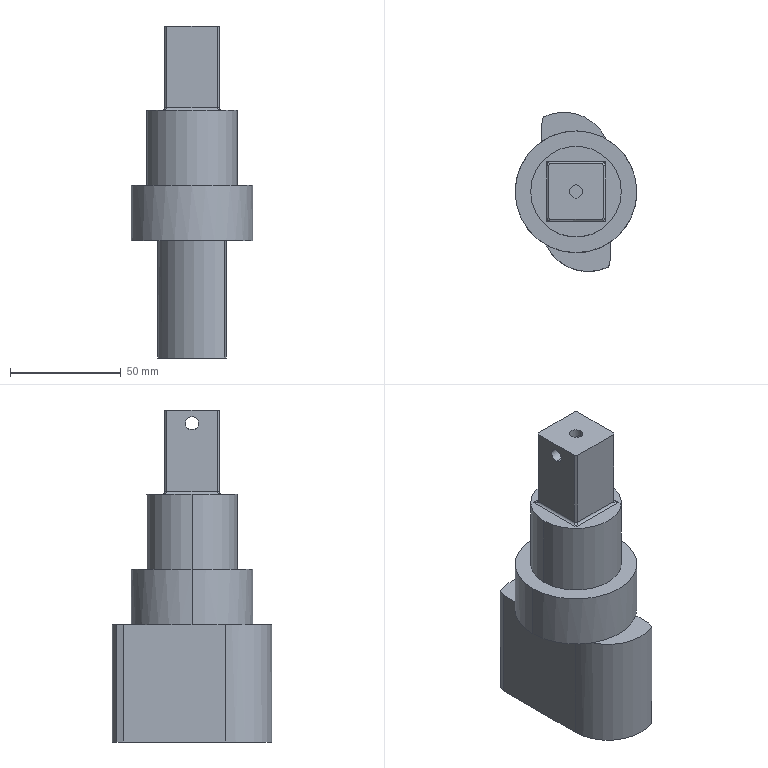Part | SolidWorks | features Boss 3, Chamfer 2, Cut 2, Extrusion 1, Fillet 1 | 1 solid | 43 faces | box 55 x 72 x 150 mm | volume 234412 mm3 | plane 21 | cylinder 18 | spline 4 | commonest cylinder face diameters 6 x8 2 x4 41 x2 42 x2 55 x2
STEP:
#1=CARTESIAN_POINT('',(-3.,0.,140.));
#2=VERTEX_POINT('',#1);
#3=CARTESIAN_POINT('',(3.,0.,140.));
#4=VERTEX_POINT('',#3);
#5=CARTESIAN_POINT('',(0.,0.,140.));
#6=DIRECTION('',(0.,0.,1.));
#7=DIRECTION('',(1.,0.,0.));
#8=AXIS2_PLACEMENT_3D('',#5,#6,#7);
#9=CIRCLE('',#8,3.);
#10=EDGE_CURVE('',#2,#4,#9,.T.);
#11=ORIENTED_EDGE('',*,*,#10,.F.);
#12=CARTESIAN_POINT('',(-3.,0.,141.));
#13=VERTEX_POINT('',#12);
#14=CARTESIAN_POINT('',(-3.,0.,140.));
#15=DIRECTION('',(0.,0.,1.));
#16=VECTOR('',#15,1000.);
#17=LINE('',#14,#16);
#18=EDGE_CURVE('',#2,#13,#17,.T.);
#19=ORIENTED_EDGE('',*,*,#18,.T.);
#20=CARTESIAN_POINT('',(0.,-3.,144.));
#21=VERTEX_POINT('',#20);
#22=CARTESIAN_POINT('',(0.,-3.,144.));
#23=CARTESIAN_POINT('',(-1.757,-3.,142.243));
#24=CARTESIAN_POINT('',(-3.,-1.757,141.));
#25=CARTESIAN_POINT('',(-3.,0.,141.));
#26=(BOUNDED_CURVE()B_SPLINE_CURVE(3,(#22,#23,#24,#25),.UNSPECIFIED.,.F.,.F.)B_SPLINE_CURVE_WITH_KNOTS((4,4),(4.712,6.283),.UNSPECIFIED.)CURVE()GEOMETRIC_REPRESENTATION_ITEM()RATIONAL_B_SPLINE_CURVE((1.,0.8047,0.8047,1.))REPRESENTATION_ITEM(''));
#27=EDGE_CURVE('',#21,#13,#26,.T.);
#28=ORIENTED_EDGE('',*,*,#27,.F.);
#29=CARTESIAN_POINT('',(3.,0.,141.));
#30=VERTEX_POINT('',#29);
#31=CARTESIAN_POINT('',(3.,0.,141.));
#32=CARTESIAN_POINT('',(3.,-1.757,141.));
#33=CARTESIAN_POINT('',(1.757,-3.,142.243));
#34=CARTESIAN_POINT('',(0.,-3.,144.));
#35=(BOUNDED_CURVE()B_SPLINE_CURVE(3,(#31,#32,#33,#34),.UNSPECIFIED.,.F.,.F.)B_SPLINE_CURVE_WITH_KNOTS((4,4),(3.142,4.712),.UNSPECIFIED.)CURVE()GEOMETRIC_REPRESENTATION_ITEM()RATIONAL_B_SPLINE_CURVE((1.,0.8047,0.8047,1.))REPRESENTATION_ITEM(''));
#36=EDGE_CURVE('',#30,#21,#35,.T.);
#37=ORIENTED_EDGE('',*,*,#36,.F.);
#38=CARTESIAN_POINT('',(3.,0.,140.));
#39=DIRECTION('',(0.,0.,1.));
#40=VECTOR('',#39,1000.);
#41=LINE('',#38,#40);
#42=EDGE_CURVE('',#4,#30,#41,.T.);
#43=ORIENTED_EDGE('',*,*,#42,.F.);
#44=EDGE_LOOP('',(#11,#19,#28,#37,#43));
#45=FACE_OUTER_BOUND('',#44,.T.);
#46=CARTESIAN_POINT('',(0.,0.,140.));
#47=DIRECTION('',(0.,0.,1.));
#48=DIRECTION('',(1.,0.,0.));
#49=AXIS2_PLACEMENT_3D('',#46,#47,#48);
#50=CYLINDRICAL_SURFACE('',#49,3.);
#51=ADVANCED_FACE('',(#45),#50,.F.);
#52=CARTESIAN_POINT('',(-3.,0.,147.));
#53=VERTEX_POINT('',#52);
#54=CARTESIAN_POINT('',(-3.,0.,147.));
#55=CARTESIAN_POINT('',(-3.,-1.757,147.));
#56=CARTESIAN_POINT('',(-1.757,-3.,145.757));
#57=CARTESIAN_POINT('',(0.,-3.,144.));
#58=(BOUNDED_CURVE()B_SPLINE_CURVE(3,(#54,#55,#56,#57),.UNSPECIFIED.,.F.,.F.)B_SPLINE_CURVE_WITH_KNOTS((4,4),(0.,1.571),.UNSPECIFIED.)CURVE()GEOMETRIC_REPRESENTATION_ITEM()RATIONAL_B_SPLINE_CURVE((1.,0.8047,0.8047,1.))REPRESENTATION_ITEM(''));
#59=EDGE_CURVE('',#53,#21,#58,.T.);
#60=ORIENTED_EDGE('',*,*,#59,.F.);
#61=CARTESIAN_POINT('',(-3.,0.,150.));
#62=VERTEX_POINT('',#61);
#63=CARTESIAN_POINT('',(-3.,0.,140.));
#64=DIRECTION('',(0.,0.,1.));
#65=VECTOR('',#64,1000.);
#66=LINE('',#63,#65);
#67=EDGE_CURVE('',#53,#62,#66,.T.);
#68=ORIENTED_EDGE('',*,*,#67,.T.);
#69=CARTESIAN_POINT('',(3.,0.,150.));
#70=VERTEX_POINT('',#69);
#71=CARTESIAN_POINT('',(0.,0.,150.));
#72=DIRECTION('',(0.,0.,1.));
#73=DIRECTION('',(1.,0.,0.));
#74=AXIS2_PLACEMENT_3D('',#71,#72,#73);
#75=CIRCLE('',#74,3.);
#76=EDGE_CURVE('',#62,#70,#75,.T.);
#77=ORIENTED_EDGE('',*,*,#76,.T.);
#78=CARTESIAN_POINT('',(3.,0.,147.));
#79=VERTEX_POINT('',#78);
#80=CARTESIAN_POINT('',(3.,0.,140.));
#81=DIRECTION('',(0.,0.,1.));
#82=VECTOR('',#81,1000.);
#83=LINE('',#80,#82);
#84=EDGE_CURVE('',#79,#70,#83,.T.);
#85=ORIENTED_EDGE('',*,*,#84,.F.);
#86=CARTESIAN_POINT('',(0.,-3.,144.));
#87=CARTESIAN_POINT('',(1.757,-3.,145.757));
#88=CARTESIAN_POINT('',(3.,-1.757,147.));
#89=CARTESIAN_POINT('',(3.,0.,147.));
#90=(BOUNDED_CURVE()B_SPLINE_CURVE(3,(#86,#87,#88,#89),.UNSPECIFIED.,.F.,.F.)B_SPLINE_CURVE_WITH_KNOTS((4,4),(1.571,3.142),.UNSPECIFIED.)CURVE()GEOMETRIC_REPRESENTATION_ITEM()RATIONAL_B_SPLINE_CURVE((1.,0.8047,0.8047,1.))REPRESENTATION_ITEM(''));
#91=EDGE_CURVE('',#21,#79,#90,.T.);
#92=ORIENTED_EDGE('',*,*,#91,.F.);
#93=EDGE_LOOP('',(#60,#68,#77,#85,#92));
#94=FACE_OUTER_BOUND('',#93,.T.);
#95=CARTESIAN_POINT('',(0.,0.,140.));
#96=DIRECTION('',(0.,0.,1.));
#97=DIRECTION('',(1.,0.,0.));
#98=AXIS2_PLACEMENT_3D('',#95,#96,#97);
#99=CYLINDRICAL_SURFACE('',#98,3.);
#100=ADVANCED_FACE('',(#94),#99,.F.);
#101=CARTESIAN_POINT('',(12.5,0.,147.));
#102=VERTEX_POINT('',#101);
#103=CARTESIAN_POINT('',(12.5,0.,141.));
#104=VERTEX_POINT('',#103);
#105=CARTESIAN_POINT('',(12.5,0.,144.));
#106=DIRECTION('',(1.,0.,0.));
#107=DIRECTION('',(0.,-1.,0.));
#108=AXIS2_PLACEMENT_3D('',#105,#106,#107);
#109=CIRCLE('',#108,3.);
#110=EDGE_CURVE('',#102,#104,#109,.T.);
#111=ORIENTED_EDGE('',*,*,#110,.T.);
#112=CARTESIAN_POINT('',(27.501,0.,141.));
#113=DIRECTION('',(-1.,0.,0.));
#114=VECTOR('',#113,1000.);
#115=LINE('',#112,#114);
#116=EDGE_CURVE('',#104,#30,#115,.T.);
#117=ORIENTED_EDGE('',*,*,#116,.T.);
#118=ORIENTED_EDGE('',*,*,#36,.T.);
#119=ORIENTED_EDGE('',*,*,#91,.T.);
#120=CARTESIAN_POINT('',(27.501,0.,147.));
#121=DIRECTION('',(-1.,0.,0.));
#122=VECTOR('',#121,1000.);
#123=LINE('',#120,#122);
#124=EDGE_CURVE('',#102,#79,#123,.T.);
#125=ORIENTED_EDGE('',*,*,#124,.F.);
#126=EDGE_LOOP('',(#111,#117,#118,#119,#125));
#127=FACE_OUTER_BOUND('',#126,.T.);
#128=CARTESIAN_POINT('',(27.501,0.,144.));
#129=DIRECTION('',(-1.,0.,0.));
#130=DIRECTION('',(0.,0.,1.));
#131=AXIS2_PLACEMENT_3D('',#128,#129,#130);
#132=CYLINDRICAL_SURFACE('',#131,3.);
#133=ADVANCED_FACE('',(#127),#132,.F.);
#134=CARTESIAN_POINT('',(20.5,0.,112.));
#135=VERTEX_POINT('',#134);
#136=CARTESIAN_POINT('',(-20.5,0.,112.));
#137=VERTEX_POINT('',#136);
#138=CARTESIAN_POINT('',(0.,0.,112.));
#139=DIRECTION('',(0.,0.,1.));
#140=DIRECTION('',(1.,0.,0.));
#141=AXIS2_PLACEMENT_3D('',#138,#139,#140);
#142=CIRCLE('',#141,20.5);
#143=EDGE_CURVE('',#135,#137,#142,.T.);
#144=ORIENTED_EDGE('',*,*,#143,.F.);
#145=CARTESIAN_POINT('',(20.5,0.,78.));
#146=VERTEX_POINT('',#145);
#147=CARTESIAN_POINT('',(20.5,0.,112.));
#148=DIRECTION('',(0.,0.,-1.));
#149=VECTOR('',#148,1000.);
#150=LINE('',#147,#149);
#151=EDGE_CURVE('',#135,#146,#150,.T.);
#152=ORIENTED_EDGE('',*,*,#151,.T.);
#153=CARTESIAN_POINT('',(-20.5,0.,78.));
#154=VERTEX_POINT('',#153);
#155=CARTESIAN_POINT('',(0.,0.,78.));
#156=DIRECTION('',(0.,0.,1.));
#157=DIRECTION('',(1.,0.,0.));
#158=AXIS2_PLACEMENT_3D('',#155,#156,#157);
#159=CIRCLE('',#158,20.5);
#160=EDGE_CURVE('',#146,#154,#159,.T.);
#161=ORIENTED_EDGE('',*,*,#160,.T.);
#162=CARTESIAN_POINT('',(-20.5,0.,112.));
#163=DIRECTION('',(0.,0.,-1.));
#164=VECTOR('',#163,1000.);
#165=LINE('',#162,#164);
#166=EDGE_CURVE('',#137,#154,#165,.T.);
#167=ORIENTED_EDGE('',*,*,#166,.F.);
#168=EDGE_LOOP('',(#144,#152,#161,#167));
#169=FACE_OUTER_BOUND('',#168,.T.);
#170=CARTESIAN_POINT('',(0.,0.,112.));
#171=DIRECTION('',(0.,0.,-1.));
#172=DIRECTION('',(-1.,0.,0.));
#173=AXIS2_PLACEMENT_3D('',#170,#171,#172);
#174=CYLINDRICAL_SURFACE('',#173,20.5);
#175=ADVANCED_FACE('',(#169),#174,.T.);
#176=CARTESIAN_POINT('',(27.5,0.,78.));
#177=VERTEX_POINT('',#176);
#178=CARTESIAN_POINT('',(-27.5,0.,78.));
#179=VERTEX_POINT('',#178);
#180=CARTESIAN_POINT('',(0.,0.,78.));
#181=DIRECTION('',(0.,0.,1.));
#182=DIRECTION('',(1.,0.,0.));
#183=AXIS2_PLACEMENT_3D('',#180,#181,#182);
#184=CIRCLE('',#183,27.5);
#185=EDGE_CURVE('',#177,#179,#184,.T.);
#186=ORIENTED_EDGE('',*,*,#185,.F.);
#187=CARTESIAN_POINT('',(27.5,0.,53.));
#188=VERTEX_POINT('',#187);
#189=CARTESIAN_POINT('',(27.5,0.,78.));
#190=DIRECTION('',(0.,0.,-1.));
#191=VECTOR('',#190,1000.);
#192=LINE('',#189,#191);
#193=EDGE_CURVE('',#177,#188,#192,.T.);
#194=ORIENTED_EDGE('',*,*,#193,.T.);
#195=CARTESIAN_POINT('',(13.491,23.963,53.));
#196=VERTEX_POINT('',#195);
#197=CARTESIAN_POINT('',(0.,0.,53.));
#198=DIRECTION('',(0.,0.,1.));
#199=DIRECTION('',(1.,0.,0.));
#200=AXIS2_PLACEMENT_3D('',#197,#198,#199);
#201=CIRCLE('',#200,27.5);
#202=EDGE_CURVE('',#188,#196,#201,.T.);
#203=ORIENTED_EDGE('',*,*,#202,.T.);
#204=CARTESIAN_POINT('',(-15.5,22.716,53.));
#205=VERTEX_POINT('',#204);
#206=CARTESIAN_POINT('',(0.,0.,53.));
#207=DIRECTION('',(0.,0.,1.));
#208=DIRECTION('',(1.,0.,0.));
#209=AXIS2_PLACEMENT_3D('',#206,#207,#208);
#210=CIRCLE('',#209,27.5);
#211=EDGE_CURVE('',#196,#205,#210,.T.);
#212=ORIENTED_EDGE('',*,*,#211,.T.);
#213=CARTESIAN_POINT('',(-27.5,0.,53.));
#214=VERTEX_POINT('',#213);
#215=CARTESIAN_POINT('',(0.,0.,53.));
#216=DIRECTION('',(0.,0.,1.));
#217=DIRECTION('',(1.,0.,0.));
#218=AXIS2_PLACEMENT_3D('',#215,#216,#217);
#219=CIRCLE('',#218,27.5);
#220=EDGE_CURVE('',#205,#214,#219,.T.);
#221=ORIENTED_EDGE('',*,*,#220,.T.);
#222=CARTESIAN_POINT('',(-27.5,0.,78.));
#223=DIRECTION('',(0.,0.,-1.));
#224=VECTOR('',#223,1000.);
#225=LINE('',#222,#224);
#226=EDGE_CURVE('',#179,#214,#225,.T.);
#227=ORIENTED_EDGE('',*,*,#226,.F.);
#228=EDGE_LOOP('',(#186,#194,#203,#212,#221,#227));
#229=FACE_OUTER_BOUND('',#228,.T.);
#230=CARTESIAN_POINT('',(0.,0.,78.));
#231=DIRECTION('',(0.,0.,-1.));
#232=DIRECTION('',(-1.,0.,0.));
#233=AXIS2_PLACEMENT_3D('',#230,#231,#232);
#234=CYLINDRICAL_SURFACE('',#233,27.5);
#235=ADVANCED_FACE('',(#229),#234,.T.);
#236=ORIENTED_EDGE('',*,*,#27,.T.);
#237=CARTESIAN_POINT('',(-12.5,0.,141.));
#238=VERTEX_POINT('',#237);
#239=CARTESIAN_POINT('',(27.501,0.,141.));
#240=DIRECTION('',(-1.,0.,0.));
#241=VECTOR('',#240,1000.);
#242=LINE('',#239,#241);
#243=EDGE_CURVE('',#13,#238,#242,.T.);
#244=ORIENTED_EDGE('',*,*,#243,.T.);
#245=CARTESIAN_POINT('',(-12.5,0.,147.));
#246=VERTEX_POINT('',#245);
#247=CARTESIAN_POINT('',(-12.5,0.,144.));
#248=DIRECTION('',(-1.,0.,0.));
#249=DIRECTION('',(0.,0.,1.));
#250=AXIS2_PLACEMENT_3D('',#247,#248,#249);
#251=CIRCLE('',#250,3.);
#252=EDGE_CURVE('',#238,#246,#251,.T.);
#253=ORIENTED_EDGE('',*,*,#252,.T.);
#254=CARTESIAN_POINT('',(27.501,0.,147.));
#255=DIRECTION('',(-1.,0.,0.));
#256=VECTOR('',#255,1000.);
#257=LINE('',#254,#256);
#258=EDGE_CURVE('',#53,#246,#257,.T.);
#259=ORIENTED_EDGE('',*,*,#258,.F.);
#260=ORIENTED_EDGE('',*,*,#59,.T.);
#261=EDGE_LOOP('',(#236,#244,#253,#259,#260));
#262=FACE_OUTER_BOUND('',#261,.T.);
#263=CARTESIAN_POINT('',(27.501,0.,144.));
#264=DIRECTION('',(-1.,0.,0.));
#265=DIRECTION('',(0.,0.,1.));
#266=AXIS2_PLACEMENT_3D('',#263,#264,#265);
#267=CYLINDRICAL_SURFACE('',#266,3.);
#268=ADVANCED_FACE('',(#262),#267,.F.);
#269=ORIENTED_EDGE('',*,*,#243,.F.);
#270=CARTESIAN_POINT('',(0.,3.,144.));
#271=VERTEX_POINT('',#270);
#272=CARTESIAN_POINT('',(-3.,0.,141.));
#273=CARTESIAN_POINT('',(-3.,1.757,141.));
#274=CARTESIAN_POINT('',(-1.757,3.,142.243));
#275=CARTESIAN_POINT('',(0.,3.,144.));
#276=(BOUNDED_CURVE()B_SPLINE_CURVE(3,(#272,#273,#274,#275),.UNSPECIFIED.,.F.,.T.)B_SPLINE_CURVE_WITH_KNOTS((4,4),(0.,1.571),.UNSPECIFIED.)CURVE()GEOMETRIC_REPRESENTATION_ITEM()RATIONAL_B_SPLINE_CURVE((1.,0.8047,0.8047,1.))REPRESENTATION_ITEM(''));
#277=EDGE_CURVE('',#13,#271,#276,.T.);
#278=ORIENTED_EDGE('',*,*,#277,.T.);
#279=CARTESIAN_POINT('',(0.,3.,144.));
#280=CARTESIAN_POINT('',(-1.757,3.,145.757));
#281=CARTESIAN_POINT('',(-3.,1.757,147.));
#282=CARTESIAN_POINT('',(-3.,0.,147.));
#283=(BOUNDED_CURVE()B_SPLINE_CURVE(3,(#279,#280,#281,#282),.UNSPECIFIED.,.F.,.F.)B_SPLINE_CURVE_WITH_KNOTS((4,4),(4.712,6.283),.UNSPECIFIED.)CURVE()GEOMETRIC_REPRESENTATION_ITEM()RATIONAL_B_SPLINE_CURVE((1.,0.8047,0.8047,1.))REPRESENTATION_ITEM(''));
#284=EDGE_CURVE('',#271,#53,#283,.T.);
#285=ORIENTED_EDGE('',*,*,#284,.T.);
#286=ORIENTED_EDGE('',*,*,#258,.T.);
#287=CARTESIAN_POINT('',(-12.5,0.,144.));
#288=DIRECTION('',(-1.,0.,0.));
#289=DIRECTION('',(0.,0.,1.));
#290=AXIS2_PLACEMENT_3D('',#287,#288,#289);
#291=CIRCLE('',#290,3.);
#292=EDGE_CURVE('',#246,#238,#291,.T.);
#293=ORIENTED_EDGE('',*,*,#292,.T.);
#294=EDGE_LOOP('',(#269,#278,#285,#286,#293));
#295=FACE_OUTER_BOUND('',#294,.T.);
#296=CARTESIAN_POINT('',(27.501,0.,144.));
#297=DIRECTION('',(-1.,0.,0.));
#298=DIRECTION('',(0.,0.,1.));
#299=AXIS2_PLACEMENT_3D('',#296,#297,#298);
#300=CYLINDRICAL_SURFACE('',#299,3.);
#301=ADVANCED_FACE('',(#295),#300,.F.);
#302=CARTESIAN_POINT('',(0.,0.,78.));
#303=DIRECTION('',(0.,0.,1.));
#304=DIRECTION('',(1.,0.,0.));
#305=AXIS2_PLACEMENT_3D('',#302,#303,#304);
#306=CIRCLE('',#305,27.5);
#307=EDGE_CURVE('',#179,#177,#306,.T.);
#308=ORIENTED_EDGE('',*,*,#307,.T.);
#309=ORIENTED_EDGE('',*,*,#185,.T.);
#310=EDGE_LOOP('',(#308,#309));
#311=FACE_OUTER_BOUND('',#310,.T.);
#312=CARTESIAN_POINT('',(0.,0.,78.));
#313=DIRECTION('',(0.,0.,1.));
#314=DIRECTION('',(1.,0.,0.));
#315=AXIS2_PLACEMENT_3D('',#312,#313,#314);
#316=CIRCLE('',#315,20.5);
#317=EDGE_CURVE('',#154,#146,#316,.T.);
#318=ORIENTED_EDGE('',*,*,#317,.F.);
#319=ORIENTED_EDGE('',*,*,#160,.F.);
#320=EDGE_LOOP('',(#318,#319));
#321=FACE_BOUND('',#320,.T.);
#322=CARTESIAN_POINT('',(0.,0.,78.));
#323=DIRECTION('',(0.,0.,1.));
#324=DIRECTION('',(1.,0.,0.));
#325=AXIS2_PLACEMENT_3D('',#322,#323,#324);
#326=PLANE('',#325);
#327=ADVANCED_FACE('',(#311,#321),#326,.T.);
#328=CARTESIAN_POINT('',(-14.63,33.912,53.));
#329=VERTEX_POINT('',#328);
#330=CARTESIAN_POINT('',(-5.5,15.,53.));
#331=DIRECTION('',(0.,0.,1.));
#332=DIRECTION('',(-1.,0.,0.));
#333=AXIS2_PLACEMENT_3D('',#330,#331,#332);
#334=CIRCLE('',#333,21.);
#335=EDGE_CURVE('',#196,#329,#334,.T.);
#336=ORIENTED_EDGE('',*,*,#335,.T.);
#337=CARTESIAN_POINT('',(-15.5,30.986,53.));
#338=VERTEX_POINT('',#337);
#339=CARTESIAN_POINT('',(-15.5,30.986,53.));
#340=DIRECTION('',(-0.2851,-0.9585,0.));
#341=VECTOR('',#340,1000.);
#342=LINE('',#339,#341);
#343=EDGE_CURVE('',#329,#338,#342,.T.);
#344=ORIENTED_EDGE('',*,*,#343,.T.);
#345=CARTESIAN_POINT('',(-15.5,-1.397,53.));
#346=DIRECTION('',(0.,-1.,0.));
#347=VECTOR('',#346,1000.);
#348=LINE('',#345,#347);
#349=EDGE_CURVE('',#338,#205,#348,.T.);
#350=ORIENTED_EDGE('',*,*,#349,.T.);
#351=ORIENTED_EDGE('',*,*,#211,.F.);
#352=EDGE_LOOP('',(#336,#344,#350,#351));
#353=FACE_OUTER_BOUND('',#352,.T.);
#354=CARTESIAN_POINT('',(-66.761,-1.397,53.));
#355=DIRECTION('',(0.,0.,-1.));
#356=DIRECTION('',(-1.,0.,0.));
#357=AXIS2_PLACEMENT_3D('',#354,#355,#356);
#358=PLANE('',#357);
#359=ADVANCED_FACE('',(#353),#358,.F.);
#360=CARTESIAN_POINT('',(-13.491,-23.963,53.));
#361=VERTEX_POINT('',#360);
#362=CARTESIAN_POINT('',(14.63,-33.912,53.));
#363=VERTEX_POINT('',#362);
#364=CARTESIAN_POINT('',(5.5,-15.,53.));
#365=DIRECTION('',(0.,0.,1.));
#366=DIRECTION('',(-1.,0.,0.));
#367=AXIS2_PLACEMENT_3D('',#364,#365,#366);
#368=CIRCLE('',#367,21.);
#369=EDGE_CURVE('',#361,#363,#368,.T.);
#370=ORIENTED_EDGE('',*,*,#369,.T.);
#371=CARTESIAN_POINT('',(15.5,-30.986,53.));
#372=VERTEX_POINT('',#371);
#373=CARTESIAN_POINT('',(15.5,-30.986,53.));
#374=DIRECTION('',(0.2851,0.9585,0.));
#375=VECTOR('',#374,1000.);
#376=LINE('',#373,#375);
#377=EDGE_CURVE('',#363,#372,#376,.T.);
#378=ORIENTED_EDGE('',*,*,#377,.T.);
#379=CARTESIAN_POINT('',(15.5,-22.716,53.));
#380=VERTEX_POINT('',#379);
#381=CARTESIAN_POINT('',(15.5,-1.397,53.));
#382=DIRECTION('',(0.,-1.,0.));
#383=VECTOR('',#382,1000.);
#384=LINE('',#381,#383);
#385=EDGE_CURVE('',#380,#372,#384,.T.);
#386=ORIENTED_EDGE('',*,*,#385,.F.);
#387=CARTESIAN_POINT('',(0.,0.,53.));
#388=DIRECTION('',(0.,0.,1.));
#389=DIRECTION('',(1.,0.,0.));
#390=AXIS2_PLACEMENT_3D('',#387,#388,#389);
#391=CIRCLE('',#390,27.5);
#392=EDGE_CURVE('',#361,#380,#391,.T.);
#393=ORIENTED_EDGE('',*,*,#392,.F.);
#394=EDGE_LOOP('',(#370,#378,#386,#393));
#395=FACE_OUTER_BOUND('',#394,.T.);
#396=CARTESIAN_POINT('',(-66.761,-1.397,53.));
#397=DIRECTION('',(0.,0.,-1.));
#398=DIRECTION('',(-1.,0.,0.));
#399=AXIS2_PLACEMENT_3D('',#396,#397,#398);
#400=PLANE('',#399);
#401=ADVANCED_FACE('',(#395),#400,.F.);
#402=CARTESIAN_POINT('',(-15.5,-15.,0.));
#403=VERTEX_POINT('',#402);
#404=CARTESIAN_POINT('',(14.63,-33.912,0.));
#405=VERTEX_POINT('',#404);
#406=CARTESIAN_POINT('',(5.5,-15.,0.));
#407=DIRECTION('',(0.,0.,1.));
#408=DIRECTION('',(-1.,0.,0.));
#409=AXIS2_PLACEMENT_3D('',#406,#407,#408);
#410=CIRCLE('',#409,21.);
#411=EDGE_CURVE('',#403,#405,#410,.T.);
#412=ORIENTED_EDGE('',*,*,#411,.T.);
#413=CARTESIAN_POINT('',(14.63,-33.912,53.));
#414=DIRECTION('',(0.,0.,1.));
#415=VECTOR('',#414,1000.);
#416=LINE('',#413,#415);
#417=EDGE_CURVE('',#405,#363,#416,.T.);
#418=ORIENTED_EDGE('',*,*,#417,.T.);
#419=ORIENTED_EDGE('',*,*,#369,.F.);
#420=CARTESIAN_POINT('',(-15.5,-15.,53.));
#421=VERTEX_POINT('',#420);
#422=CARTESIAN_POINT('',(5.5,-15.,53.));
#423=DIRECTION('',(0.,0.,1.));
#424=DIRECTION('',(-1.,0.,0.));
#425=AXIS2_PLACEMENT_3D('',#422,#423,#424);
#426=CIRCLE('',#425,21.);
#427=EDGE_CURVE('',#421,#361,#426,.T.);
#428=ORIENTED_EDGE('',*,*,#427,.F.);
#429=CARTESIAN_POINT('',(-15.5,-15.,53.));
#430=DIRECTION('',(0.,0.,-1.));
#431=VECTOR('',#430,1000.);
#432=LINE('',#429,#431);
#433=EDGE_CURVE('',#421,#403,#432,.T.);
#434=ORIENTED_EDGE('',*,*,#433,.T.);
#435=EDGE_LOOP('',(#412,#418,#419,#428,#434));
#436=FACE_OUTER_BOUND('',#435,.T.);
#437=CARTESIAN_POINT('',(5.5,-15.,53.));
#438=DIRECTION('',(0.,0.,-1.));
#439=DIRECTION('',(-1.,0.,0.));
#440=AXIS2_PLACEMENT_3D('',#437,#438,#439);
#441=CYLINDRICAL_SURFACE('',#440,21.);
#442=ADVANCED_FACE('',(#436),#441,.T.);
#443=ORIENTED_EDGE('',*,*,#385,.T.);
#444=CARTESIAN_POINT('',(15.5,-30.986,0.));
#445=VERTEX_POINT('',#444);
#446=CARTESIAN_POINT('',(15.5,-30.986,0.));
#447=DIRECTION('',(0.,0.,-1.));
#448=VECTOR('',#447,1000.);
#449=LINE('',#446,#448);
#450=EDGE_CURVE('',#372,#445,#449,.T.);
#451=ORIENTED_EDGE('',*,*,#450,.T.);
#452=CARTESIAN_POINT('',(15.5,15.,0.));
#453=VERTEX_POINT('',#452);
#454=CARTESIAN_POINT('',(15.5,-1.397,0.));
#455=DIRECTION('',(0.,-1.,0.));
#456=VECTOR('',#455,1000.);
#457=LINE('',#454,#456);
#458=EDGE_CURVE('',#453,#445,#457,.T.);
#459=ORIENTED_EDGE('',*,*,#458,.F.);
#460=CARTESIAN_POINT('',(15.5,15.,53.));
#461=VERTEX_POINT('',#460);
#462=CARTESIAN_POINT('',(15.5,15.,53.));
#463=DIRECTION('',(0.,0.,-1.));
#464=VECTOR('',#463,1000.);
#465=LINE('',#462,#464);
#466=EDGE_CURVE('',#461,#453,#465,.T.);
#467=ORIENTED_EDGE('',*,*,#466,.F.);
#468=CARTESIAN_POINT('',(15.5,-1.397,53.));
#469=DIRECTION('',(0.,-1.,0.));
#470=VECTOR('',#469,1000.);
#471=LINE('',#468,#470);
#472=EDGE_CURVE('',#461,#380,#471,.T.);
#473=ORIENTED_EDGE('',*,*,#472,.T.);
#474=EDGE_LOOP('',(#443,#451,#459,#467,#473));
#475=FACE_OUTER_BOUND('',#474,.T.);
#476=CARTESIAN_POINT('',(15.5,-1.397,53.));
#477=DIRECTION('',(1.,0.,0.));
#478=DIRECTION('',(0.,0.,-1.));
#479=AXIS2_PLACEMENT_3D('',#476,#477,#478);
#480=PLANE('',#479);
#481=ADVANCED_FACE('',(#475),#480,.T.);
#482=CARTESIAN_POINT('',(-14.63,33.912,0.));
#483=VERTEX_POINT('',#482);
#484=CARTESIAN_POINT('',(-5.5,15.,0.));
#485=DIRECTION('',(0.,0.,1.));
#486=DIRECTION('',(-1.,0.,0.));
#487=AXIS2_PLACEMENT_3D('',#484,#485,#486);
#488=CIRCLE('',#487,21.);
#489=EDGE_CURVE('',#453,#483,#488,.T.);
#490=ORIENTED_EDGE('',*,*,#489,.T.);
#491=CARTESIAN_POINT('',(-14.63,33.912,53.));
#492=DIRECTION('',(0.,0.,1.));
#493=VECTOR('',#492,1000.);
#494=LINE('',#491,#493);
#495=EDGE_CURVE('',#483,#329,#494,.T.);
#496=ORIENTED_EDGE('',*,*,#495,.T.);
#497=ORIENTED_EDGE('',*,*,#335,.F.);
#498=CARTESIAN_POINT('',(-5.5,15.,53.));
#499=DIRECTION('',(0.,0.,1.));
#500=DIRECTION('',(-1.,0.,0.));
#501=AXIS2_PLACEMENT_3D('',#498,#499,#500);
#502=CIRCLE('',#501,21.);
#503=EDGE_CURVE('',#461,#196,#502,.T.);
#504=ORIENTED_EDGE('',*,*,#503,.F.);
#505=ORIENTED_EDGE('',*,*,#466,.T.);
#506=EDGE_LOOP('',(#490,#496,#497,#504,#505));
#507=FACE_OUTER_BOUND('',#506,.T.);
#508=CARTESIAN_POINT('',(-5.5,15.,53.));
#509=DIRECTION('',(0.,0.,-1.));
#510=DIRECTION('',(-1.,0.,0.));
#511=AXIS2_PLACEMENT_3D('',#508,#509,#510);
#512=CYLINDRICAL_SURFACE('',#511,21.);
#513=ADVANCED_FACE('',(#507),#512,.T.);
#514=ORIENTED_EDGE('',*,*,#349,.F.);
#515=CARTESIAN_POINT('',(-15.5,30.986,0.));
#516=VERTEX_POINT('',#515);
#517=CARTESIAN_POINT('',(-15.5,30.986,53.));
#518=DIRECTION('',(0.,0.,-1.));
#519=VECTOR('',#518,1000.);
#520=LINE('',#517,#519);
#521=EDGE_CURVE('',#338,#516,#520,.T.);
#522=ORIENTED_EDGE('',*,*,#521,.T.);
#523=CARTESIAN_POINT('',(-15.5,-1.397,0.));
#524=DIRECTION('',(0.,-1.,0.));
#525=VECTOR('',#524,1000.);
#526=LINE('',#523,#525);
#527=EDGE_CURVE('',#516,#403,#526,.T.);
#528=ORIENTED_EDGE('',*,*,#527,.T.);
#529=ORIENTED_EDGE('',*,*,#433,.F.);
#530=CARTESIAN_POINT('',(-15.5,-1.397,53.));
#531=DIRECTION('',(0.,-1.,0.));
#532=VECTOR('',#531,1000.);
#533=LINE('',#530,#532);
#534=EDGE_CURVE('',#205,#421,#533,.T.);
#535=ORIENTED_EDGE('',*,*,#534,.F.);
#536=EDGE_LOOP('',(#514,#522,#528,#529,#535));
#537=FACE_OUTER_BOUND('',#536,.T.);
#538=CARTESIAN_POINT('',(-15.5,-1.397,53.));
#539=DIRECTION('',(1.,0.,0.));
#540=DIRECTION('',(0.,1.,0.));
#541=AXIS2_PLACEMENT_3D('',#538,#539,#540);
#542=PLANE('',#541);
#543=ADVANCED_FACE('',(#537),#542,.F.);
#544=ORIENTED_EDGE('',*,*,#458,.T.);
#545=CARTESIAN_POINT('',(16.9,-26.279,0.));
#546=DIRECTION('',(-0.2851,-0.9585,0.));
#547=VECTOR('',#546,1000.);
#548=LINE('',#545,#547);
#549=EDGE_CURVE('',#445,#405,#548,.T.);
#550=ORIENTED_EDGE('',*,*,#549,.T.);
#551=ORIENTED_EDGE('',*,*,#411,.F.);
#552=ORIENTED_EDGE('',*,*,#527,.F.);
#553=CARTESIAN_POINT('',(-28.514,-12.772,0.));
#554=DIRECTION('',(0.2851,0.9585,0.));
#555=VECTOR('',#554,1000.);
#556=LINE('',#553,#555);
#557=EDGE_CURVE('',#516,#483,#556,.T.);
#558=ORIENTED_EDGE('',*,*,#557,.T.);
#559=ORIENTED_EDGE('',*,*,#489,.F.);
#560=EDGE_LOOP('',(#544,#550,#551,#552,#558,#559));
#561=FACE_OUTER_BOUND('',#560,.T.);
#562=CARTESIAN_POINT('',(-66.761,-1.397,0.));
#563=DIRECTION('',(0.,0.,-1.));
#564=DIRECTION('',(-1.,0.,0.));
#565=AXIS2_PLACEMENT_3D('',#562,#563,#564);
#566=PLANE('',#565);
#567=ADVANCED_FACE('',(#561),#566,.T.);
#568=ORIENTED_EDGE('',*,*,#534,.T.);
#569=ORIENTED_EDGE('',*,*,#427,.T.);
#570=CARTESIAN_POINT('',(0.,0.,53.));
#571=DIRECTION('',(0.,0.,1.));
#572=DIRECTION('',(1.,0.,0.));
#573=AXIS2_PLACEMENT_3D('',#570,#571,#572);
#574=CIRCLE('',#573,27.5);
#575=EDGE_CURVE('',#214,#361,#574,.T.);
#576=ORIENTED_EDGE('',*,*,#575,.F.);
#577=ORIENTED_EDGE('',*,*,#220,.F.);
#578=EDGE_LOOP('',(#568,#569,#576,#577));
#579=FACE_OUTER_BOUND('',#578,.T.);
#580=CARTESIAN_POINT('',(0.,0.,53.));
#581=DIRECTION('',(0.,0.,1.));
#582=DIRECTION('',(1.,0.,0.));
#583=AXIS2_PLACEMENT_3D('',#580,#581,#582);
#584=PLANE('',#583);
#585=ADVANCED_FACE('',(#579),#584,.F.);
#586=ORIENTED_EDGE('',*,*,#193,.F.);
#587=ORIENTED_EDGE('',*,*,#307,.F.);
#588=ORIENTED_EDGE('',*,*,#226,.T.);
#589=ORIENTED_EDGE('',*,*,#575,.T.);
#590=ORIENTED_EDGE('',*,*,#392,.T.);
#591=CARTESIAN_POINT('',(0.,0.,53.));
#592=DIRECTION('',(0.,0.,1.));
#593=DIRECTION('',(1.,0.,0.));
#594=AXIS2_PLACEMENT_3D('',#591,#592,#593);
#595=CIRCLE('',#594,27.5);
#596=EDGE_CURVE('',#380,#188,#595,.T.);
#597=ORIENTED_EDGE('',*,*,#596,.T.);
#598=EDGE_LOOP('',(#586,#587,#588,#589,#590,#597));
#599=FACE_OUTER_BOUND('',#598,.T.);
#600=CARTESIAN_POINT('',(0.,0.,78.));
#601=DIRECTION('',(0.,0.,-1.));
#602=DIRECTION('',(-1.,0.,0.));
#603=AXIS2_PLACEMENT_3D('',#600,#601,#602);
#604=CYLINDRICAL_SURFACE('',#603,27.5);
#605=ADVANCED_FACE('',(#599),#604,.T.);
#606=ORIENTED_EDGE('',*,*,#472,.F.);
#607=ORIENTED_EDGE('',*,*,#503,.T.);
#608=ORIENTED_EDGE('',*,*,#202,.F.);
#609=ORIENTED_EDGE('',*,*,#596,.F.);
#610=EDGE_LOOP('',(#606,#607,#608,#609));
#611=FACE_OUTER_BOUND('',#610,.T.);
#612=CARTESIAN_POINT('',(0.,0.,53.));
#613=DIRECTION('',(0.,0.,1.));
#614=DIRECTION('',(1.,0.,0.));
#615=AXIS2_PLACEMENT_3D('',#612,#613,#614);
#616=PLANE('',#615);
#617=ADVANCED_FACE('',(#611),#616,.F.);
#618=ORIENTED_EDGE('',*,*,#151,.F.);
#619=CARTESIAN_POINT('',(0.,0.,112.));
#620=DIRECTION('',(0.,0.,1.));
#621=DIRECTION('',(1.,0.,0.));
#622=AXIS2_PLACEMENT_3D('',#619,#620,#621);
#623=CIRCLE('',#622,20.5);
#624=EDGE_CURVE('',#137,#135,#623,.T.);
#625=ORIENTED_EDGE('',*,*,#624,.F.);
#626=ORIENTED_EDGE('',*,*,#166,.T.);
#627=ORIENTED_EDGE('',*,*,#317,.T.);
#628=EDGE_LOOP('',(#618,#625,#626,#627));
#629=FACE_OUTER_BOUND('',#628,.T.);
#630=CARTESIAN_POINT('',(0.,0.,112.));
#631=DIRECTION('',(0.,0.,-1.));
#632=DIRECTION('',(-1.,0.,0.));
#633=AXIS2_PLACEMENT_3D('',#630,#631,#632);
#634=CYLINDRICAL_SURFACE('',#633,20.5);
#635=ADVANCED_FACE('',(#629),#634,.T.);
#636=CARTESIAN_POINT('',(13.5,13.5,112.));
#637=VERTEX_POINT('',#636);
#638=CARTESIAN_POINT('',(13.5,-13.5,112.));
#639=VERTEX_POINT('',#638);
#640=CARTESIAN_POINT('',(13.5,0.,112.));
#641=DIRECTION('',(0.,-1.,0.));
#642=VECTOR('',#641,1000.);
#643=LINE('',#640,#642);
#644=EDGE_CURVE('',#637,#639,#643,.T.);
#645=ORIENTED_EDGE('',*,*,#644,.T.);
#646=CARTESIAN_POINT('',(-13.5,-13.5,112.));
#647=VERTEX_POINT('',#646);
#648=CARTESIAN_POINT('',(-12.5,-13.5,112.));
#649=DIRECTION('',(-1.,0.,0.));
#650=VECTOR('',#649,1000.);
#651=LINE('',#648,#650);
#652=EDGE_CURVE('',#639,#647,#651,.T.);
#653=ORIENTED_EDGE('',*,*,#652,.T.);
#654=CARTESIAN_POINT('',(-13.5,13.5,112.));
#655=VERTEX_POINT('',#654);
#656=CARTESIAN_POINT('',(-13.5,12.5,112.));
#657=DIRECTION('',(0.,1.,0.));
#658=VECTOR('',#657,1000.);
#659=LINE('',#656,#658);
#660=EDGE_CURVE('',#647,#655,#659,.T.);
#661=ORIENTED_EDGE('',*,*,#660,.T.);
#662=CARTESIAN_POINT('',(0.,13.5,112.));
#663=DIRECTION('',(1.,0.,0.));
#664=VECTOR('',#663,1000.);
#665=LINE('',#662,#664);
#666=EDGE_CURVE('',#655,#637,#665,.T.);
#667=ORIENTED_EDGE('',*,*,#666,.T.);
#668=EDGE_LOOP('',(#645,#653,#661,#667));
#669=FACE_BOUND('',#668,.T.);
#670=ORIENTED_EDGE('',*,*,#624,.T.);
#671=ORIENTED_EDGE('',*,*,#143,.T.);
#672=EDGE_LOOP('',(#670,#671));
#673=FACE_OUTER_BOUND('',#672,.T.);
#674=CARTESIAN_POINT('',(0.,0.,112.));
#675=DIRECTION('',(0.,0.,1.));
#676=DIRECTION('',(1.,0.,0.));
#677=AXIS2_PLACEMENT_3D('',#674,#675,#676);
#678=PLANE('',#677);
#679=ADVANCED_FACE('',(#669,#673),#678,.T.);
#680=CARTESIAN_POINT('',(-11.5,-12.5,113.));
#681=VERTEX_POINT('',#680);
#682=CARTESIAN_POINT('',(11.5,-12.5,113.));
#683=VERTEX_POINT('',#682);
#684=CARTESIAN_POINT('',(12.5,-12.5,113.));
#685=DIRECTION('',(1.,0.,0.));
#686=VECTOR('',#685,1000.);
#687=LINE('',#684,#686);
#688=EDGE_CURVE('',#681,#683,#687,.T.);
#689=ORIENTED_EDGE('',*,*,#688,.T.);
#690=CARTESIAN_POINT('',(11.5,-12.5,150.));
#691=VERTEX_POINT('',#690);
#692=CARTESIAN_POINT('',(11.5,-12.5,150.));
#693=DIRECTION('',(0.,0.,1.));
#694=VECTOR('',#693,1000.);
#695=LINE('',#692,#694);
#696=EDGE_CURVE('',#683,#691,#695,.T.);
#697=ORIENTED_EDGE('',*,*,#696,.T.);
#698=CARTESIAN_POINT('',(-11.5,-12.5,150.));
#699=VERTEX_POINT('',#698);
#700=CARTESIAN_POINT('',(-66.761,-12.5,150.));
#701=DIRECTION('',(-1.,0.,0.));
#702=VECTOR('',#701,1000.);
#703=LINE('',#700,#702);
#704=EDGE_CURVE('',#691,#699,#703,.T.);
#705=ORIENTED_EDGE('',*,*,#704,.T.);
#706=CARTESIAN_POINT('',(-11.5,-12.5,150.));
#707=DIRECTION('',(0.,0.,-1.));
#708=VECTOR('',#707,1000.);
#709=LINE('',#706,#708);
#710=EDGE_CURVE('',#699,#681,#709,.T.);
#711=ORIENTED_EDGE('',*,*,#710,.T.);
#712=EDGE_LOOP('',(#689,#697,#705,#711));
#713=FACE_OUTER_BOUND('',#712,.T.);
#714=CARTESIAN_POINT('',(-66.761,-12.5,150.));
#715=DIRECTION('',(0.,-1.,0.));
#716=DIRECTION('',(1.,0.,0.));
#717=AXIS2_PLACEMENT_3D('',#714,#715,#716);
#718=PLANE('',#717);
#719=ADVANCED_FACE('',(#713),#718,.T.);
#720=ORIENTED_EDGE('',*,*,#110,.F.);
#721=CARTESIAN_POINT('',(12.5,0.,144.));
#722=DIRECTION('',(1.,0.,0.));
#723=DIRECTION('',(0.,-1.,0.));
#724=AXIS2_PLACEMENT_3D('',#721,#722,#723);
#725=CIRCLE('',#724,3.);
#726=EDGE_CURVE('',#104,#102,#725,.T.);
#727=ORIENTED_EDGE('',*,*,#726,.F.);
#728=EDGE_LOOP('',(#720,#727));
#729=FACE_BOUND('',#728,.T.);
#730=CARTESIAN_POINT('',(12.5,-11.5,113.));
#731=VERTEX_POINT('',#730);
#732=CARTESIAN_POINT('',(12.5,11.5,113.));
#733=VERTEX_POINT('',#732);
#734=CARTESIAN_POINT('',(12.5,-1.397,113.));
#735=DIRECTION('',(0.,1.,0.));
#736=VECTOR('',#735,1000.);
#737=LINE('',#734,#736);
#738=EDGE_CURVE('',#731,#733,#737,.T.);
#739=ORIENTED_EDGE('',*,*,#738,.T.);
#740=CARTESIAN_POINT('',(12.5,11.5,150.));
#741=VERTEX_POINT('',#740);
#742=CARTESIAN_POINT('',(12.5,11.5,150.));
#743=DIRECTION('',(0.,0.,1.));
#744=VECTOR('',#743,1000.);
#745=LINE('',#742,#744);
#746=EDGE_CURVE('',#733,#741,#745,.T.);
#747=ORIENTED_EDGE('',*,*,#746,.T.);
#748=CARTESIAN_POINT('',(12.5,-11.5,150.));
#749=VERTEX_POINT('',#748);
#750=CARTESIAN_POINT('',(12.5,-1.397,150.));
#751=DIRECTION('',(0.,1.,0.));
#752=VECTOR('',#751,1000.);
#753=LINE('',#750,#752);
#754=EDGE_CURVE('',#749,#741,#753,.T.);
#755=ORIENTED_EDGE('',*,*,#754,.F.);
#756=CARTESIAN_POINT('',(12.5,-11.5,113.));
#757=DIRECTION('',(0.,0.,-1.));
#758=VECTOR('',#757,1000.);
#759=LINE('',#756,#758);
#760=EDGE_CURVE('',#749,#731,#759,.T.);
#761=ORIENTED_EDGE('',*,*,#760,.T.);
#762=EDGE_LOOP('',(#739,#747,#755,#761));
#763=FACE_OUTER_BOUND('',#762,.T.);
#764=CARTESIAN_POINT('',(12.5,-1.397,150.));
#765=DIRECTION('',(-1.,0.,0.));
#766=DIRECTION('',(0.,-1.,0.));
#767=AXIS2_PLACEMENT_3D('',#764,#765,#766);
#768=PLANE('',#767);
#769=ADVANCED_FACE('',(#729,#763),#768,.F.);
#770=CARTESIAN_POINT('',(11.5,12.5,113.));
#771=VERTEX_POINT('',#770);
#772=CARTESIAN_POINT('',(-11.5,12.5,113.));
#773=VERTEX_POINT('',#772);
#774=CARTESIAN_POINT('',(-66.761,12.5,113.));
#775=DIRECTION('',(-1.,0.,0.));
#776=VECTOR('',#775,1000.);
#777=LINE('',#774,#776);
#778=EDGE_CURVE('',#771,#773,#777,.T.);
#779=ORIENTED_EDGE('',*,*,#778,.T.);
#780=CARTESIAN_POINT('',(-11.5,12.5,150.));
#781=VERTEX_POINT('',#780);
#782=CARTESIAN_POINT('',(-11.5,12.5,150.));
#783=DIRECTION('',(0.,0.,1.));
#784=VECTOR('',#783,1000.);
#785=LINE('',#782,#784);
#786=EDGE_CURVE('',#773,#781,#785,.T.);
#787=ORIENTED_EDGE('',*,*,#786,.T.);
#788=CARTESIAN_POINT('',(11.5,12.5,150.));
#789=VERTEX_POINT('',#788);
#790=CARTESIAN_POINT('',(-66.761,12.5,150.));
#791=DIRECTION('',(-1.,0.,0.));
#792=VECTOR('',#791,1000.);
#793=LINE('',#790,#792);
#794=EDGE_CURVE('',#789,#781,#793,.T.);
#795=ORIENTED_EDGE('',*,*,#794,.F.);
#796=CARTESIAN_POINT('',(11.5,12.5,150.));
#797=DIRECTION('',(0.,0.,-1.));
#798=VECTOR('',#797,1000.);
#799=LINE('',#796,#798);
#800=EDGE_CURVE('',#789,#771,#799,.T.);
#801=ORIENTED_EDGE('',*,*,#800,.T.);
#802=EDGE_LOOP('',(#779,#787,#795,#801));
#803=FACE_OUTER_BOUND('',#802,.T.);
#804=CARTESIAN_POINT('',(-66.761,12.5,150.));
#805=DIRECTION('',(0.,-1.,0.));
#806=DIRECTION('',(1.,0.,0.));
#807=AXIS2_PLACEMENT_3D('',#804,#805,#806);
#808=PLANE('',#807);
#809=ADVANCED_FACE('',(#803),#808,.F.);
#810=ORIENTED_EDGE('',*,*,#292,.F.);
#811=ORIENTED_EDGE('',*,*,#252,.F.);
#812=EDGE_LOOP('',(#810,#811));
#813=FACE_BOUND('',#812,.T.);
#814=CARTESIAN_POINT('',(-12.5,-11.5,150.));
#815=VERTEX_POINT('',#814);
#816=CARTESIAN_POINT('',(-12.5,11.5,150.));
#817=VERTEX_POINT('',#816);
#818=CARTESIAN_POINT('',(-12.5,-1.397,150.));
#819=DIRECTION('',(0.,1.,0.));
#820=VECTOR('',#819,1000.);
#821=LINE('',#818,#820);
#822=EDGE_CURVE('',#815,#817,#821,.T.);
#823=ORIENTED_EDGE('',*,*,#822,.T.);
#824=CARTESIAN_POINT('',(-12.5,11.5,113.));
#825=VERTEX_POINT('',#824);
#826=CARTESIAN_POINT('',(-12.5,11.5,113.));
#827=DIRECTION('',(0.,0.,-1.));
#828=VECTOR('',#827,1000.);
#829=LINE('',#826,#828);
#830=EDGE_CURVE('',#817,#825,#829,.T.);
#831=ORIENTED_EDGE('',*,*,#830,.T.);
#832=CARTESIAN_POINT('',(-12.5,-11.5,113.));
#833=VERTEX_POINT('',#832);
#834=CARTESIAN_POINT('',(-12.5,-12.5,113.));
#835=DIRECTION('',(0.,-1.,0.));
#836=VECTOR('',#835,1000.);
#837=LINE('',#834,#836);
#838=EDGE_CURVE('',#825,#833,#837,.T.);
#839=ORIENTED_EDGE('',*,*,#838,.T.);
#840=CARTESIAN_POINT('',(-12.5,-11.5,150.));
#841=DIRECTION('',(0.,0.,1.));
#842=VECTOR('',#841,1000.);
#843=LINE('',#840,#842);
#844=EDGE_CURVE('',#833,#815,#843,.T.);
#845=ORIENTED_EDGE('',*,*,#844,.T.);
#846=EDGE_LOOP('',(#823,#831,#839,#845));
#847=FACE_OUTER_BOUND('',#846,.T.);
#848=CARTESIAN_POINT('',(-12.5,-1.397,150.));
#849=DIRECTION('',(-1.,0.,0.));
#850=DIRECTION('',(0.,0.,1.));
#851=AXIS2_PLACEMENT_3D('',#848,#849,#850);
#852=PLANE('',#851);
#853=ADVANCED_FACE('',(#813,#847),#852,.T.);
#854=CARTESIAN_POINT('',(0.,0.,150.));
#855=DIRECTION('',(0.,0.,1.));
#856=DIRECTION('',(1.,0.,0.));
#857=AXIS2_PLACEMENT_3D('',#854,#855,#856);
#858=CIRCLE('',#857,3.);
#859=EDGE_CURVE('',#70,#62,#858,.T.);
#860=ORIENTED_EDGE('',*,*,#859,.F.);
#861=ORIENTED_EDGE('',*,*,#76,.F.);
#862=EDGE_LOOP('',(#860,#861));
#863=FACE_BOUND('',#862,.T.);
#864=ORIENTED_EDGE('',*,*,#794,.T.);
#865=CARTESIAN_POINT('',(-12.5,11.5,150.));
#866=DIRECTION('',(-0.7071,-0.7071,0.));
#867=VECTOR('',#866,1000.);
#868=LINE('',#865,#867);
#869=EDGE_CURVE('',#781,#817,#868,.T.);
#870=ORIENTED_EDGE('',*,*,#869,.T.);
#871=ORIENTED_EDGE('',*,*,#822,.F.);
#872=CARTESIAN_POINT('',(-11.5,-12.5,150.));
#873=DIRECTION('',(0.7071,-0.7071,0.));
#874=VECTOR('',#873,1000.);
#875=LINE('',#872,#874);
#876=EDGE_CURVE('',#815,#699,#875,.T.);
#877=ORIENTED_EDGE('',*,*,#876,.T.);
#878=ORIENTED_EDGE('',*,*,#704,.F.);
#879=CARTESIAN_POINT('',(12.5,-11.5,150.));
#880=DIRECTION('',(0.7071,0.7071,0.));
#881=VECTOR('',#880,1000.);
#882=LINE('',#879,#881);
#883=EDGE_CURVE('',#691,#749,#882,.T.);
#884=ORIENTED_EDGE('',*,*,#883,.T.);
#885=ORIENTED_EDGE('',*,*,#754,.T.);
#886=CARTESIAN_POINT('',(11.5,12.5,150.));
#887=DIRECTION('',(-0.7071,0.7071,0.));
#888=VECTOR('',#887,1000.);
#889=LINE('',#886,#888);
#890=EDGE_CURVE('',#741,#789,#889,.T.);
#891=ORIENTED_EDGE('',*,*,#890,.T.);
#892=EDGE_LOOP('',(#864,#870,#871,#877,#878,#884,#885,#891));
#893=FACE_OUTER_BOUND('',#892,.T.);
#894=CARTESIAN_POINT('',(-66.761,-1.397,150.));
#895=DIRECTION('',(0.,0.,-1.));
#896=DIRECTION('',(-1.,0.,0.));
#897=AXIS2_PLACEMENT_3D('',#894,#895,#896);
#898=PLANE('',#897);
#899=ADVANCED_FACE('',(#863,#893),#898,.F.);
#900=ORIENTED_EDGE('',*,*,#377,.F.);
#901=ORIENTED_EDGE('',*,*,#417,.F.);
#902=ORIENTED_EDGE('',*,*,#549,.F.);
#903=ORIENTED_EDGE('',*,*,#450,.F.);
#904=EDGE_LOOP('',(#900,#901,#902,#903));
#905=FACE_OUTER_BOUND('',#904,.T.);
#906=CARTESIAN_POINT('',(15.5,-30.986,53.));
#907=DIRECTION('',(-0.9585,0.2851,0.));
#908=DIRECTION('',(-0.2851,-0.9585,0.));
#909=AXIS2_PLACEMENT_3D('',#906,#907,#908);
#910=PLANE('',#909);
#911=ADVANCED_FACE('',(#905),#910,.F.);
#912=ORIENTED_EDGE('',*,*,#343,.F.);
#913=ORIENTED_EDGE('',*,*,#495,.F.);
#914=ORIENTED_EDGE('',*,*,#557,.F.);
#915=ORIENTED_EDGE('',*,*,#521,.F.);
#916=EDGE_LOOP('',(#912,#913,#914,#915));
#917=FACE_OUTER_BOUND('',#916,.T.);
#918=CARTESIAN_POINT('',(-15.5,30.986,53.));
#919=DIRECTION('',(0.9585,-0.2851,0.));
#920=DIRECTION('',(0.2851,0.9585,0.));
#921=AXIS2_PLACEMENT_3D('',#918,#919,#920);
#922=PLANE('',#921);
#923=ADVANCED_FACE('',(#917),#922,.F.);
#924=ORIENTED_EDGE('',*,*,#116,.F.);
#925=ORIENTED_EDGE('',*,*,#726,.T.);
#926=ORIENTED_EDGE('',*,*,#124,.T.);
#927=CARTESIAN_POINT('',(3.,0.,147.));
#928=CARTESIAN_POINT('',(3.,1.757,147.));
#929=CARTESIAN_POINT('',(1.757,3.,145.757));
#930=CARTESIAN_POINT('',(0.,3.,144.));
#931=(BOUNDED_CURVE()B_SPLINE_CURVE(3,(#927,#928,#929,#930),.UNSPECIFIED.,.F.,.T.)B_SPLINE_CURVE_WITH_KNOTS((4,4),(3.142,4.712),.UNSPECIFIED.)CURVE()GEOMETRIC_REPRESENTATION_ITEM()RATIONAL_B_SPLINE_CURVE((1.,0.8047,0.8047,1.))REPRESENTATION_ITEM(''));
#932=EDGE_CURVE('',#79,#271,#931,.T.);
#933=ORIENTED_EDGE('',*,*,#932,.T.);
#934=CARTESIAN_POINT('',(0.,3.,144.));
#935=CARTESIAN_POINT('',(1.757,3.,142.243));
#936=CARTESIAN_POINT('',(3.,1.757,141.));
#937=CARTESIAN_POINT('',(3.,0.,141.));
#938=(BOUNDED_CURVE()B_SPLINE_CURVE(3,(#934,#935,#936,#937),.UNSPECIFIED.,.F.,.T.)B_SPLINE_CURVE_WITH_KNOTS((4,4),(1.571,3.142),.UNSPECIFIED.)CURVE()GEOMETRIC_REPRESENTATION_ITEM()RATIONAL_B_SPLINE_CURVE((1.,0.8047,0.8047,1.))REPRESENTATION_ITEM(''));
#939=EDGE_CURVE('',#271,#30,#938,.T.);
#940=ORIENTED_EDGE('',*,*,#939,.T.);
#941=EDGE_LOOP('',(#924,#925,#926,#933,#940));
#942=FACE_OUTER_BOUND('',#941,.T.);
#943=CARTESIAN_POINT('',(27.501,0.,144.));
#944=DIRECTION('',(-1.,0.,0.));
#945=DIRECTION('',(0.,0.,1.));
#946=AXIS2_PLACEMENT_3D('',#943,#944,#945);
#947=CYLINDRICAL_SURFACE('',#946,3.);
#948=ADVANCED_FACE('',(#942),#947,.F.);
#949=ORIENTED_EDGE('',*,*,#67,.F.);
#950=ORIENTED_EDGE('',*,*,#284,.F.);
#951=ORIENTED_EDGE('',*,*,#932,.F.);
#952=ORIENTED_EDGE('',*,*,#84,.T.);
#953=ORIENTED_EDGE('',*,*,#859,.T.);
#954=EDGE_LOOP('',(#949,#950,#951,#952,#953));
#955=FACE_OUTER_BOUND('',#954,.T.);
#956=CARTESIAN_POINT('',(0.,0.,140.));
#957=DIRECTION('',(0.,0.,1.));
#958=DIRECTION('',(1.,0.,0.));
#959=AXIS2_PLACEMENT_3D('',#956,#957,#958);
#960=CYLINDRICAL_SURFACE('',#959,3.);
#961=ADVANCED_FACE('',(#955),#960,.F.);
#962=ORIENTED_EDGE('',*,*,#18,.F.);
#963=CARTESIAN_POINT('',(0.,0.,140.));
#964=DIRECTION('',(0.,0.,1.));
#965=DIRECTION('',(1.,0.,0.));
#966=AXIS2_PLACEMENT_3D('',#963,#964,#965);
#967=CIRCLE('',#966,3.);
#968=EDGE_CURVE('',#4,#2,#967,.T.);
#969=ORIENTED_EDGE('',*,*,#968,.F.);
#970=ORIENTED_EDGE('',*,*,#42,.T.);
#971=ORIENTED_EDGE('',*,*,#939,.F.);
#972=ORIENTED_EDGE('',*,*,#277,.F.);
#973=EDGE_LOOP('',(#962,#969,#970,#971,#972));
#974=FACE_OUTER_BOUND('',#973,.T.);
#975=CARTESIAN_POINT('',(0.,0.,140.));
#976=DIRECTION('',(0.,0.,1.));
#977=DIRECTION('',(1.,0.,0.));
#978=AXIS2_PLACEMENT_3D('',#975,#976,#977);
#979=CYLINDRICAL_SURFACE('',#978,3.);
#980=ADVANCED_FACE('',(#974),#979,.F.);
#981=ORIENTED_EDGE('',*,*,#968,.T.);
#982=ORIENTED_EDGE('',*,*,#10,.T.);
#983=EDGE_LOOP('',(#981,#982));
#984=FACE_OUTER_BOUND('',#983,.T.);
#985=CARTESIAN_POINT('',(0.,0.,140.));
#986=DIRECTION('',(0.,0.,1.));
#987=DIRECTION('',(1.,0.,0.));
#988=AXIS2_PLACEMENT_3D('',#985,#986,#987);
#989=PLANE('',#988);
#990=ADVANCED_FACE('',(#984),#989,.T.);
#991=ORIENTED_EDGE('',*,*,#666,.F.);
#992=CARTESIAN_POINT('',(-13.5,13.5,112.));
#993=CARTESIAN_POINT('',(-13.157,13.329,112.));
#994=CARTESIAN_POINT('',(-12.868,13.18,112.044));
#995=CARTESIAN_POINT('',(-12.515,13.003,112.13));
#996=CARTESIAN_POINT('',(-12.411,12.952,112.162));
#997=CARTESIAN_POINT('',(-12.275,12.885,112.211));
#998=CARTESIAN_POINT('',(-12.233,12.864,112.228));
#999=CARTESIAN_POINT('',(-12.175,12.836,112.252));
#1000=CARTESIAN_POINT('',(-12.148,12.822,112.265));
#1001=CARTESIAN_POINT('',(-12.118,12.807,112.279));
#1002=CARTESIAN_POINT('',(-12.103,12.8,112.286));
#1003=CARTESIAN_POINT('',(-12.097,12.797,112.289));
#1004=CARTESIAN_POINT('',(-12.093,12.795,112.291));
#1005=CARTESIAN_POINT('',(-12.092,12.794,112.291));
#1006=CARTESIAN_POINT('',(-11.887,12.691,112.394));
#1007=CARTESIAN_POINT('',(-11.736,12.617,112.513));
#1008=CARTESIAN_POINT('',(-11.54,12.521,112.757));
#1009=CARTESIAN_POINT('',(-11.494,12.5,112.882));
#1010=CARTESIAN_POINT('',(-11.5,12.5,113.));
#1011=B_SPLINE_CURVE_WITH_KNOTS('',3,(#992,#993,#994,#995,#996,#997,#998,#999,#1000,#1001,#1002,#1003,#1004,#1005,#1006,#1007,#1008,#1009,#1010),.UNSPECIFIED.,.F.,.F.,(4,2,2,2,1,1,1,2,2,2,4),(0.,0.25,0.375,0.4375,0.4687,0.4844,0.4922,0.4961,0.5,0.75,1.),.UNSPECIFIED.);
#1012=EDGE_CURVE('',#655,#773,#1011,.T.);
#1013=ORIENTED_EDGE('',*,*,#1012,.T.);
#1014=ORIENTED_EDGE('',*,*,#778,.F.);
#1015=CARTESIAN_POINT('',(11.5,12.5,113.));
#1016=CARTESIAN_POINT('',(11.494,12.5,112.882));
#1017=CARTESIAN_POINT('',(11.54,12.521,112.757));
#1018=CARTESIAN_POINT('',(11.687,12.593,112.574));
#1019=CARTESIAN_POINT('',(11.749,12.623,112.514));
#1020=CARTESIAN_POINT('',(11.862,12.679,112.427));
#1021=CARTESIAN_POINT('',(11.903,12.7,112.399));
#1022=CARTESIAN_POINT('',(11.969,12.733,112.358));
#1023=CARTESIAN_POINT('',(12.003,12.75,112.338));
#1024=CARTESIAN_POINT('',(12.045,12.771,112.315));
#1025=CARTESIAN_POINT('',(12.067,12.782,112.304));
#1026=CARTESIAN_POINT('',(12.076,12.787,112.299));
#1027=CARTESIAN_POINT('',(12.083,12.79,112.296));
#1028=CARTESIAN_POINT('',(12.087,12.792,112.294));
#1029=CARTESIAN_POINT('',(12.216,12.857,112.229));
#1030=CARTESIAN_POINT('',(12.398,12.944,112.158));
#1031=CARTESIAN_POINT('',(12.868,13.18,112.044));
#1032=CARTESIAN_POINT('',(13.157,13.329,112.));
#1033=CARTESIAN_POINT('',(13.5,13.5,112.));
#1034=B_SPLINE_CURVE_WITH_KNOTS('',3,(#1015,#1016,#1017,#1018,#1019,#1020,#1021,#1022,#1023,#1024,#1025,#1026,#1027,#1028,#1029,#1030,#1031,#1032,#1033),.UNSPECIFIED.,.F.,.F.,(4,2,2,2,1,1,1,2,2,2,4),(0.,0.25,0.375,0.4375,0.4688,0.4844,0.4922,0.4961,0.5,0.75,1.),.UNSPECIFIED.);
#1035=EDGE_CURVE('',#771,#637,#1034,.T.);
#1036=ORIENTED_EDGE('',*,*,#1035,.T.);
#1037=EDGE_LOOP('',(#991,#1013,#1014,#1036));
#1038=FACE_OUTER_BOUND('',#1037,.T.);
#1039=CARTESIAN_POINT('',(0.,13.5,113.));
#1040=DIRECTION('',(1.,0.,0.));
#1041=DIRECTION('',(0.,1.,0.));
#1042=AXIS2_PLACEMENT_3D('',#1039,#1040,#1041);
#1043=CYLINDRICAL_SURFACE('',#1042,1.);
#1044=ADVANCED_FACE('',(#1038),#1043,.F.);
#1045=ORIENTED_EDGE('',*,*,#838,.F.);
#1046=CARTESIAN_POINT('',(-12.5,11.5,113.));
#1047=CARTESIAN_POINT('',(-12.5,11.494,112.882));
#1048=CARTESIAN_POINT('',(-12.521,11.54,112.757));
#1049=CARTESIAN_POINT('',(-12.593,11.687,112.574));
#1050=CARTESIAN_POINT('',(-12.623,11.749,112.514));
#1051=CARTESIAN_POINT('',(-12.679,11.862,112.427));
#1052=CARTESIAN_POINT('',(-12.7,11.903,112.399));
#1053=CARTESIAN_POINT('',(-12.733,11.969,112.358));
#1054=CARTESIAN_POINT('',(-12.75,12.003,112.338));
#1055=CARTESIAN_POINT('',(-12.771,12.045,112.315));
#1056=CARTESIAN_POINT('',(-12.782,12.067,112.304));
#1057=CARTESIAN_POINT('',(-12.787,12.076,112.299));
#1058=CARTESIAN_POINT('',(-12.79,12.083,112.296));
#1059=CARTESIAN_POINT('',(-12.792,12.087,112.294));
#1060=CARTESIAN_POINT('',(-12.857,12.216,112.229));
#1061=CARTESIAN_POINT('',(-12.944,12.398,112.158));
#1062=CARTESIAN_POINT('',(-13.18,12.868,112.044));
#1063=CARTESIAN_POINT('',(-13.329,13.157,112.));
#1064=CARTESIAN_POINT('',(-13.5,13.5,112.));
#1065=B_SPLINE_CURVE_WITH_KNOTS('',3,(#1046,#1047,#1048,#1049,#1050,#1051,#1052,#1053,#1054,#1055,#1056,#1057,#1058,#1059,#1060,#1061,#1062,#1063,#1064),.UNSPECIFIED.,.F.,.F.,(4,2,2,2,1,1,1,2,2,2,4),(0.,0.25,0.375,0.4375,0.4687,0.4844,0.4922,0.4961,0.5,0.75,1.),.UNSPECIFIED.);
#1066=EDGE_CURVE('',#825,#655,#1065,.T.);
#1067=ORIENTED_EDGE('',*,*,#1066,.T.);
#1068=ORIENTED_EDGE('',*,*,#660,.F.);
#1069=CARTESIAN_POINT('',(-13.5,-13.5,112.));
#1070=CARTESIAN_POINT('',(-13.329,-13.157,112.));
#1071=CARTESIAN_POINT('',(-13.18,-12.868,112.044));
#1072=CARTESIAN_POINT('',(-13.003,-12.515,112.13));
#1073=CARTESIAN_POINT('',(-12.952,-12.411,112.162));
#1074=CARTESIAN_POINT('',(-12.885,-12.275,112.211));
#1075=CARTESIAN_POINT('',(-12.864,-12.233,112.228));
#1076=CARTESIAN_POINT('',(-12.836,-12.175,112.252));
#1077=CARTESIAN_POINT('',(-12.822,-12.148,112.265));
#1078=CARTESIAN_POINT('',(-12.807,-12.118,112.279));
#1079=CARTESIAN_POINT('',(-12.8,-12.103,112.286));
#1080=CARTESIAN_POINT('',(-12.797,-12.097,112.289));
#1081=CARTESIAN_POINT('',(-12.795,-12.093,112.291));
#1082=CARTESIAN_POINT('',(-12.794,-12.092,112.291));
#1083=CARTESIAN_POINT('',(-12.691,-11.887,112.394));
#1084=CARTESIAN_POINT('',(-12.617,-11.736,112.513));
#1085=CARTESIAN_POINT('',(-12.521,-11.54,112.757));
#1086=CARTESIAN_POINT('',(-12.5,-11.494,112.882));
#1087=CARTESIAN_POINT('',(-12.5,-11.5,113.));
#1088=B_SPLINE_CURVE_WITH_KNOTS('',3,(#1069,#1070,#1071,#1072,#1073,#1074,#1075,#1076,#1077,#1078,#1079,#1080,#1081,#1082,#1083,#1084,#1085,#1086,#1087),.UNSPECIFIED.,.F.,.F.,(4,2,2,2,1,1,1,2,2,2,4),(0.,0.25,0.375,0.4375,0.4688,0.4844,0.4922,0.4961,0.5,0.75,1.),.UNSPECIFIED.);
#1089=EDGE_CURVE('',#647,#833,#1088,.T.);
#1090=ORIENTED_EDGE('',*,*,#1089,.T.);
#1091=EDGE_LOOP('',(#1045,#1067,#1068,#1090));
#1092=FACE_OUTER_BOUND('',#1091,.T.);
#1093=CARTESIAN_POINT('',(-13.5,-1.397,113.));
#1094=DIRECTION('',(0.,1.,0.));
#1095=DIRECTION('',(0.,0.,1.));
#1096=AXIS2_PLACEMENT_3D('',#1093,#1094,#1095);
#1097=CYLINDRICAL_SURFACE('',#1096,1.);
#1098=ADVANCED_FACE('',(#1092),#1097,.F.);
#1099=ORIENTED_EDGE('',*,*,#644,.F.);
#1100=CARTESIAN_POINT('',(13.5,13.5,112.));
#1101=CARTESIAN_POINT('',(13.329,13.157,112.));
#1102=CARTESIAN_POINT('',(13.18,12.868,112.044));
#1103=CARTESIAN_POINT('',(13.003,12.515,112.13));
#1104=CARTESIAN_POINT('',(12.952,12.411,112.162));
#1105=CARTESIAN_POINT('',(12.885,12.275,112.211));
#1106=CARTESIAN_POINT('',(12.864,12.233,112.228));
#1107=CARTESIAN_POINT('',(12.836,12.175,112.252));
#1108=CARTESIAN_POINT('',(12.822,12.148,112.265));
#1109=CARTESIAN_POINT('',(12.807,12.118,112.279));
#1110=CARTESIAN_POINT('',(12.8,12.103,112.286));
#1111=CARTESIAN_POINT('',(12.797,12.097,112.289));
#1112=CARTESIAN_POINT('',(12.795,12.093,112.291));
#1113=CARTESIAN_POINT('',(12.794,12.092,112.291));
#1114=CARTESIAN_POINT('',(12.691,11.887,112.394));
#1115=CARTESIAN_POINT('',(12.617,11.736,112.513));
#1116=CARTESIAN_POINT('',(12.521,11.54,112.757));
#1117=CARTESIAN_POINT('',(12.5,11.494,112.882));
#1118=CARTESIAN_POINT('',(12.5,11.5,113.));
#1119=B_SPLINE_CURVE_WITH_KNOTS('',3,(#1100,#1101,#1102,#1103,#1104,#1105,#1106,#1107,#1108,#1109,#1110,#1111,#1112,#1113,#1114,#1115,#1116,#1117,#1118),.UNSPECIFIED.,.F.,.F.,(4,2,2,2,1,1,1,2,2,2,4),(0.,0.25,0.375,0.4375,0.4687,0.4844,0.4922,0.4961,0.5,0.75,1.),.UNSPECIFIED.);
#1120=EDGE_CURVE('',#637,#733,#1119,.T.);
#1121=ORIENTED_EDGE('',*,*,#1120,.T.);
#1122=ORIENTED_EDGE('',*,*,#738,.F.);
#1123=CARTESIAN_POINT('',(12.5,-11.5,113.));
#1124=CARTESIAN_POINT('',(12.5,-11.494,112.882));
#1125=CARTESIAN_POINT('',(12.521,-11.54,112.757));
#1126=CARTESIAN_POINT('',(12.593,-11.687,112.574));
#1127=CARTESIAN_POINT('',(12.623,-11.749,112.514));
#1128=CARTESIAN_POINT('',(12.679,-11.862,112.427));
#1129=CARTESIAN_POINT('',(12.7,-11.903,112.399));
#1130=CARTESIAN_POINT('',(12.733,-11.969,112.358));
#1131=CARTESIAN_POINT('',(12.75,-12.003,112.338));
#1132=CARTESIAN_POINT('',(12.771,-12.045,112.315));
#1133=CARTESIAN_POINT('',(12.782,-12.067,112.304));
#1134=CARTESIAN_POINT('',(12.787,-12.076,112.299));
#1135=CARTESIAN_POINT('',(12.79,-12.083,112.296));
#1136=CARTESIAN_POINT('',(12.792,-12.087,112.294));
#1137=CARTESIAN_POINT('',(12.857,-12.216,112.229));
#1138=CARTESIAN_POINT('',(12.944,-12.398,112.158));
#1139=CARTESIAN_POINT('',(13.18,-12.868,112.044));
#1140=CARTESIAN_POINT('',(13.329,-13.157,112.));
#1141=CARTESIAN_POINT('',(13.5,-13.5,112.));
#1142=B_SPLINE_CURVE_WITH_KNOTS('',3,(#1123,#1124,#1125,#1126,#1127,#1128,#1129,#1130,#1131,#1132,#1133,#1134,#1135,#1136,#1137,#1138,#1139,#1140,#1141),.UNSPECIFIED.,.F.,.F.,(4,2,2,2,1,1,1,2,2,2,4),(0.,0.25,0.375,0.4375,0.4687,0.4844,0.4922,0.4961,0.5,0.75,1.),.UNSPECIFIED.);
#1143=EDGE_CURVE('',#731,#639,#1142,.T.);
#1144=ORIENTED_EDGE('',*,*,#1143,.T.);
#1145=EDGE_LOOP('',(#1099,#1121,#1122,#1144));
#1146=FACE_OUTER_BOUND('',#1145,.T.);
#1147=CARTESIAN_POINT('',(13.5,0.,113.));
#1148=DIRECTION('',(0.,-1.,0.));
#1149=DIRECTION('',(1.,0.,0.));
#1150=AXIS2_PLACEMENT_3D('',#1147,#1148,#1149);
#1151=CYLINDRICAL_SURFACE('',#1150,1.);
#1152=ADVANCED_FACE('',(#1146),#1151,.F.);
#1153=ORIENTED_EDGE('',*,*,#652,.F.);
#1154=CARTESIAN_POINT('',(13.5,-13.5,112.));
#1155=CARTESIAN_POINT('',(13.157,-13.329,112.));
#1156=CARTESIAN_POINT('',(12.868,-13.18,112.044));
#1157=CARTESIAN_POINT('',(12.515,-13.003,112.13));
#1158=CARTESIAN_POINT('',(12.411,-12.952,112.162));
#1159=CARTESIAN_POINT('',(12.275,-12.885,112.211));
#1160=CARTESIAN_POINT('',(12.233,-12.864,112.228));
#1161=CARTESIAN_POINT('',(12.175,-12.836,112.252));
#1162=CARTESIAN_POINT('',(12.148,-12.822,112.265));
#1163=CARTESIAN_POINT('',(12.118,-12.807,112.279));
#1164=CARTESIAN_POINT('',(12.103,-12.8,112.286));
#1165=CARTESIAN_POINT('',(12.097,-12.797,112.289));
#1166=CARTESIAN_POINT('',(12.093,-12.795,112.291));
#1167=CARTESIAN_POINT('',(12.092,-12.794,112.291));
#1168=CARTESIAN_POINT('',(11.887,-12.691,112.394));
#1169=CARTESIAN_POINT('',(11.736,-12.617,112.513));
#1170=CARTESIAN_POINT('',(11.54,-12.521,112.757));
#1171=CARTESIAN_POINT('',(11.494,-12.5,112.882));
#1172=CARTESIAN_POINT('',(11.5,-12.5,113.));
#1173=B_SPLINE_CURVE_WITH_KNOTS('',3,(#1154,#1155,#1156,#1157,#1158,#1159,#1160,#1161,#1162,#1163,#1164,#1165,#1166,#1167,#1168,#1169,#1170,#1171,#1172),.UNSPECIFIED.,.F.,.F.,(4,2,2,2,1,1,1,2,2,2,4),(0.,0.25,0.375,0.4375,0.4687,0.4844,0.4922,0.4961,0.5,0.75,1.),.UNSPECIFIED.);
#1174=EDGE_CURVE('',#639,#683,#1173,.T.);
#1175=ORIENTED_EDGE('',*,*,#1174,.T.);
#1176=ORIENTED_EDGE('',*,*,#688,.F.);
#1177=CARTESIAN_POINT('',(-11.5,-12.5,113.));
#1178=CARTESIAN_POINT('',(-11.494,-12.5,112.882));
#1179=CARTESIAN_POINT('',(-11.54,-12.521,112.757));
#1180=CARTESIAN_POINT('',(-11.687,-12.593,112.574));
#1181=CARTESIAN_POINT('',(-11.749,-12.623,112.514));
#1182=CARTESIAN_POINT('',(-11.862,-12.679,112.427));
#1183=CARTESIAN_POINT('',(-11.903,-12.7,112.399));
#1184=CARTESIAN_POINT('',(-11.969,-12.733,112.358));
#1185=CARTESIAN_POINT('',(-12.003,-12.75,112.338));
#1186=CARTESIAN_POINT('',(-12.045,-12.771,112.315));
#1187=CARTESIAN_POINT('',(-12.067,-12.782,112.304));
#1188=CARTESIAN_POINT('',(-12.076,-12.787,112.299));
#1189=CARTESIAN_POINT('',(-12.083,-12.79,112.296));
#1190=CARTESIAN_POINT('',(-12.087,-12.792,112.294));
#1191=CARTESIAN_POINT('',(-12.216,-12.857,112.229));
#1192=CARTESIAN_POINT('',(-12.398,-12.944,112.158));
#1193=CARTESIAN_POINT('',(-12.868,-13.18,112.044));
#1194=CARTESIAN_POINT('',(-13.157,-13.329,112.));
#1195=CARTESIAN_POINT('',(-13.5,-13.5,112.));
#1196=B_SPLINE_CURVE_WITH_KNOTS('',3,(#1177,#1178,#1179,#1180,#1181,#1182,#1183,#1184,#1185,#1186,#1187,#1188,#1189,#1190,#1191,#1192,#1193,#1194,#1195),.UNSPECIFIED.,.F.,.F.,(4,2,2,2,1,1,1,2,2,2,4),(0.,0.25,0.375,0.4375,0.4688,0.4844,0.4922,0.4961,0.5,0.75,1.),.UNSPECIFIED.);
#1197=EDGE_CURVE('',#681,#647,#1196,.T.);
#1198=ORIENTED_EDGE('',*,*,#1197,.T.);
#1199=EDGE_LOOP('',(#1153,#1175,#1176,#1198));
#1200=FACE_OUTER_BOUND('',#1199,.T.);
#1201=CARTESIAN_POINT('',(-66.761,-13.5,113.));
#1202=DIRECTION('',(-1.,0.,0.));
#1203=DIRECTION('',(0.,-1.,0.));
#1204=AXIS2_PLACEMENT_3D('',#1201,#1202,#1203);
#1205=CYLINDRICAL_SURFACE('',#1204,1.);
#1206=ADVANCED_FACE('',(#1200),#1205,.F.);
#1207=ORIENTED_EDGE('',*,*,#869,.F.);
#1208=ORIENTED_EDGE('',*,*,#786,.F.);
#1209=CARTESIAN_POINT('',(-12.5,11.5,113.));
#1210=CARTESIAN_POINT('',(-11.5,12.5,113.));
#1211=B_SPLINE_CURVE_WITH_KNOTS('',1,(#1209,#1210),.UNSPECIFIED.,.F.,.F.,(2,2),(0.,1.),.UNSPECIFIED.);
#1212=EDGE_CURVE('',#825,#773,#1211,.T.);
#1213=ORIENTED_EDGE('',*,*,#1212,.F.);
#1214=ORIENTED_EDGE('',*,*,#830,.F.);
#1215=EDGE_LOOP('',(#1207,#1208,#1213,#1214));
#1216=FACE_OUTER_BOUND('',#1215,.T.);
#1217=CARTESIAN_POINT('',(-12.5,11.5,150.));
#1218=DIRECTION('',(-0.7071,0.7071,0.));
#1219=DIRECTION('',(-0.7071,-0.7071,0.));
#1220=AXIS2_PLACEMENT_3D('',#1217,#1218,#1219);
#1221=PLANE('',#1220);
#1222=ADVANCED_FACE('',(#1216),#1221,.T.);
#1223=ORIENTED_EDGE('',*,*,#1212,.T.);
#1224=ORIENTED_EDGE('',*,*,#1012,.F.);
#1225=ORIENTED_EDGE('',*,*,#1066,.F.);
#1226=EDGE_LOOP('',(#1223,#1224,#1225));
#1227=FACE_OUTER_BOUND('',#1226,.T.);
#1228=CARTESIAN_POINT('',(-12.5,11.5,113.));
#1229=CARTESIAN_POINT('',(-12.486,11.472,112.466));
#1230=CARTESIAN_POINT('',(-12.966,12.431,111.986));
#1231=CARTESIAN_POINT('',(-13.5,13.5,112.));
#1232=CARTESIAN_POINT('',(-11.5,12.5,113.));
#1233=CARTESIAN_POINT('',(-11.472,12.486,112.466));
#1234=CARTESIAN_POINT('',(-12.431,12.966,111.986));
#1235=CARTESIAN_POINT('',(-13.5,13.5,112.));
#1236=B_SPLINE_SURFACE_WITH_KNOTS('',1,3,((#1228,#1229,#1230,#1231),(#1232,#1233,#1234,#1235)),.UNSPECIFIED.,.F.,.F.,.F.,(2,2),(4,4),(0.,1.),(3.142,4.712),.UNSPECIFIED.);
#1237=ADVANCED_FACE('',(#1227),#1236,.T.);
#1238=ORIENTED_EDGE('',*,*,#890,.F.);
#1239=ORIENTED_EDGE('',*,*,#746,.F.);
#1240=CARTESIAN_POINT('',(11.5,12.5,113.));
#1241=CARTESIAN_POINT('',(12.5,11.5,113.));
#1242=B_SPLINE_CURVE_WITH_KNOTS('',1,(#1240,#1241),.UNSPECIFIED.,.F.,.F.,(2,2),(0.,1.),.UNSPECIFIED.);
#1243=EDGE_CURVE('',#771,#733,#1242,.T.);
#1244=ORIENTED_EDGE('',*,*,#1243,.F.);
#1245=ORIENTED_EDGE('',*,*,#800,.F.);
#1246=EDGE_LOOP('',(#1238,#1239,#1244,#1245));
#1247=FACE_OUTER_BOUND('',#1246,.T.);
#1248=CARTESIAN_POINT('',(11.5,12.5,150.));
#1249=DIRECTION('',(-0.7071,-0.7071,0.));
#1250=DIRECTION('',(0.7071,-0.7071,0.));
#1251=AXIS2_PLACEMENT_3D('',#1248,#1249,#1250);
#1252=PLANE('',#1251);
#1253=ADVANCED_FACE('',(#1247),#1252,.F.);
#1254=ORIENTED_EDGE('',*,*,#1120,.F.);
#1255=ORIENTED_EDGE('',*,*,#1035,.F.);
#1256=ORIENTED_EDGE('',*,*,#1243,.T.);
#1257=EDGE_LOOP('',(#1254,#1255,#1256));
#1258=FACE_OUTER_BOUND('',#1257,.T.);
#1259=CARTESIAN_POINT('',(11.5,12.5,113.));
#1260=CARTESIAN_POINT('',(11.472,12.486,112.466));
#1261=CARTESIAN_POINT('',(12.431,12.966,111.986));
#1262=CARTESIAN_POINT('',(13.5,13.5,112.));
#1263=CARTESIAN_POINT('',(12.5,11.5,113.));
#1264=CARTESIAN_POINT('',(12.486,11.472,112.466));
#1265=CARTESIAN_POINT('',(12.966,12.431,111.986));
#1266=CARTESIAN_POINT('',(13.5,13.5,112.));
#1267=B_SPLINE_SURFACE_WITH_KNOTS('',1,3,((#1259,#1260,#1261,#1262),(#1263,#1264,#1265,#1266)),.UNSPECIFIED.,.F.,.F.,.F.,(2,2),(4,4),(0.,1.),(0.,1.571),.UNSPECIFIED.);
#1268=ADVANCED_FACE('',(#1258),#1267,.T.);
#1269=ORIENTED_EDGE('',*,*,#883,.F.);
#1270=ORIENTED_EDGE('',*,*,#696,.F.);
#1271=CARTESIAN_POINT('',(12.5,-11.5,113.));
#1272=CARTESIAN_POINT('',(11.5,-12.5,113.));
#1273=B_SPLINE_CURVE_WITH_KNOTS('',1,(#1271,#1272),.UNSPECIFIED.,.F.,.F.,(2,2),(0.,1.),.UNSPECIFIED.);
#1274=EDGE_CURVE('',#731,#683,#1273,.T.);
#1275=ORIENTED_EDGE('',*,*,#1274,.F.);
#1276=ORIENTED_EDGE('',*,*,#760,.F.);
#1277=EDGE_LOOP('',(#1269,#1270,#1275,#1276));
#1278=FACE_OUTER_BOUND('',#1277,.T.);
#1279=CARTESIAN_POINT('',(12.5,-11.5,150.));
#1280=DIRECTION('',(0.7071,-0.7071,0.));
#1281=DIRECTION('',(0.7071,0.7071,0.));
#1282=AXIS2_PLACEMENT_3D('',#1279,#1280,#1281);
#1283=PLANE('',#1282);
#1284=ADVANCED_FACE('',(#1278),#1283,.T.);
#1285=ORIENTED_EDGE('',*,*,#1174,.F.);
#1286=ORIENTED_EDGE('',*,*,#1143,.F.);
#1287=ORIENTED_EDGE('',*,*,#1274,.T.);
#1288=EDGE_LOOP('',(#1285,#1286,#1287));
#1289=FACE_OUTER_BOUND('',#1288,.T.);
#1290=CARTESIAN_POINT('',(12.5,-11.5,113.));
#1291=CARTESIAN_POINT('',(12.486,-11.472,112.466));
#1292=CARTESIAN_POINT('',(12.966,-12.431,111.986));
#1293=CARTESIAN_POINT('',(13.5,-13.5,112.));
#1294=CARTESIAN_POINT('',(11.5,-12.5,113.));
#1295=CARTESIAN_POINT('',(11.472,-12.486,112.466));
#1296=CARTESIAN_POINT('',(12.431,-12.966,111.986));
#1297=CARTESIAN_POINT('',(13.5,-13.5,112.));
#1298=B_SPLINE_SURFACE_WITH_KNOTS('',1,3,((#1290,#1291,#1292,#1293),(#1294,#1295,#1296,#1297)),.UNSPECIFIED.,.F.,.F.,.F.,(2,2),(4,4),(0.,1.),(0.,1.571),.UNSPECIFIED.);
#1299=ADVANCED_FACE('',(#1289),#1298,.T.);
#1300=ORIENTED_EDGE('',*,*,#876,.F.);
#1301=ORIENTED_EDGE('',*,*,#844,.F.);
#1302=CARTESIAN_POINT('',(-11.5,-12.5,113.));
#1303=CARTESIAN_POINT('',(-12.5,-11.5,113.));
#1304=B_SPLINE_CURVE_WITH_KNOTS('',1,(#1302,#1303),.UNSPECIFIED.,.F.,.F.,(2,2),(0.,1.),.UNSPECIFIED.);
#1305=EDGE_CURVE('',#681,#833,#1304,.T.);
#1306=ORIENTED_EDGE('',*,*,#1305,.F.);
#1307=ORIENTED_EDGE('',*,*,#710,.F.);
#1308=EDGE_LOOP('',(#1300,#1301,#1306,#1307));
#1309=FACE_OUTER_BOUND('',#1308,.T.);
#1310=CARTESIAN_POINT('',(-11.5,-12.5,150.));
#1311=DIRECTION('',(0.7071,0.7071,0.));
#1312=DIRECTION('',(-0.7071,0.7071,0.));
#1313=AXIS2_PLACEMENT_3D('',#1310,#1311,#1312);
#1314=PLANE('',#1313);
#1315=ADVANCED_FACE('',(#1309),#1314,.F.);
#1316=ORIENTED_EDGE('',*,*,#1305,.T.);
#1317=ORIENTED_EDGE('',*,*,#1089,.F.);
#1318=ORIENTED_EDGE('',*,*,#1197,.F.);
#1319=EDGE_LOOP('',(#1316,#1317,#1318));
#1320=FACE_OUTER_BOUND('',#1319,.T.);
#1321=CARTESIAN_POINT('',(-11.5,-12.5,113.));
#1322=CARTESIAN_POINT('',(-11.472,-12.486,112.466));
#1323=CARTESIAN_POINT('',(-12.431,-12.966,111.986));
#1324=CARTESIAN_POINT('',(-13.5,-13.5,112.));
#1325=CARTESIAN_POINT('',(-12.5,-11.5,113.));
#1326=CARTESIAN_POINT('',(-12.486,-11.472,112.466));
#1327=CARTESIAN_POINT('',(-12.966,-12.431,111.986));
#1328=CARTESIAN_POINT('',(-13.5,-13.5,112.));
#1329=B_SPLINE_SURFACE_WITH_KNOTS('',1,3,((#1321,#1322,#1323,#1324),(#1325,#1326,#1327,#1328)),.UNSPECIFIED.,.F.,.F.,.F.,(2,2),(4,4),(0.,1.),(3.142,4.712),.UNSPECIFIED.);
#1330=ADVANCED_FACE('',(#1320),#1329,.T.);
#1331=CLOSED_SHELL('',(#51,#100,#133,#175,#235,#268,#301,#327,#359,#401,#442,#481,#513,#543,#567,#585,#605,#617,#635,#679,#719,#769,#809,#853,#899,#911,#923,#948,#961,#980,#990,#1044,#1098,#1152,#1206,#1222,#1237,#1253,#1268,#1284,#1299,#1315,#1330));
#1332=MANIFOLD_SOLID_BREP('',#1331);
#1333=CARTESIAN_POINT('',(0.,0.,0.));
#1334=DIRECTION('',(0.,0.,1.));
#1335=DIRECTION('',(1.,0.,0.));
#1336=AXIS2_PLACEMENT_3D('',#1333,#1334,#1335);
#1337=(LENGTH_UNIT()NAMED_UNIT(*)SI_UNIT(.MILLI.,.METRE.));
#1338=UNCERTAINTY_MEASURE_WITH_UNIT(LENGTH_MEASURE(0.00001),#1337,'','');
#1339=(NAMED_UNIT(*)PLANE_ANGLE_UNIT()SI_UNIT($,.RADIAN.));
#1340=(NAMED_UNIT(*)SI_UNIT($,.STERADIAN.)SOLID_ANGLE_UNIT());
#1341=(GEOMETRIC_REPRESENTATION_CONTEXT(3)GLOBAL_UNCERTAINTY_ASSIGNED_CONTEXT((#1338))GLOBAL_UNIT_ASSIGNED_CONTEXT((#1337,#1339,#1340))REPRESENTATION_CONTEXT('',''));
#1342=ADVANCED_BREP_SHAPE_REPRESENTATION('',(#1332,#1336),#1341);